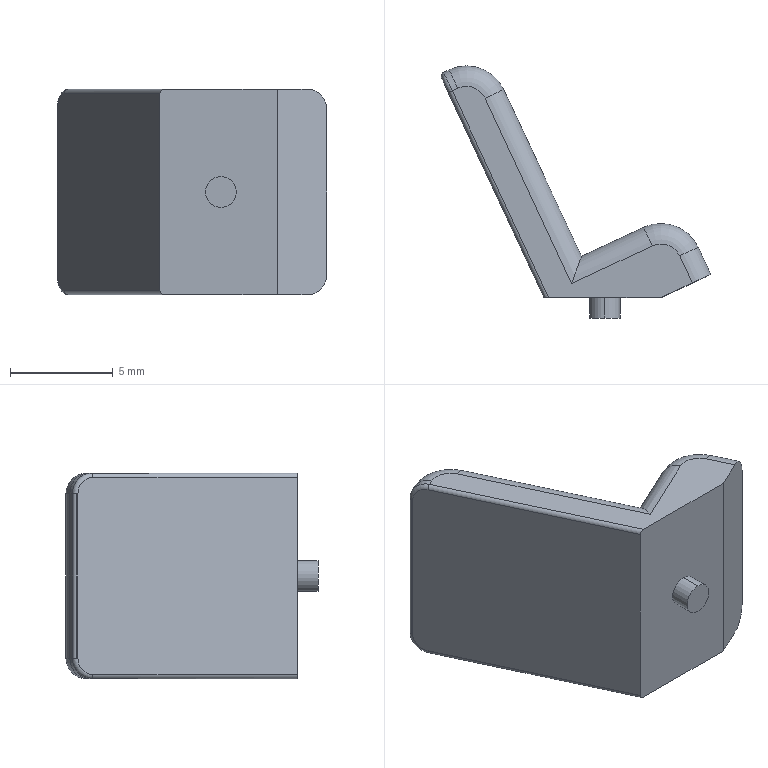Part | SolidWorks | features Fillet 2, Extrusion 1, ICE 1 | 1 solid | 32 faces | box 13.131 x 12.274 x 10 mm | volume 457.95 mm3 | cylinder 16 | plane 10 | torus 6 | commonest cylinder face diameters 2 x8 0.4 x4 1.5 x2 4 x2
STEP:
#1=CARTESIAN_POINT('',(2.965,-1.,-0.75));
#2=VERTEX_POINT('',#1);
#3=CARTESIAN_POINT('',(2.965,-1.,0.75));
#4=VERTEX_POINT('',#3);
#5=CARTESIAN_POINT('',(2.965,-1.,0.));
#6=DIRECTION('',(0.,-1.,0.));
#7=DIRECTION('',(0.,0.,-1.));
#8=AXIS2_PLACEMENT_3D('',#5,#6,#7);
#9=CIRCLE('',#8,0.75);
#10=EDGE_CURVE('',#2,#4,#9,.T.);
#11=ORIENTED_EDGE('',*,*,#10,.F.);
#12=CARTESIAN_POINT('',(2.965,0.,-0.75));
#13=VERTEX_POINT('',#12);
#14=CARTESIAN_POINT('',(2.965,-1.,-0.75));
#15=DIRECTION('',(0.,1.,0.));
#16=VECTOR('',#15,1000.);
#17=LINE('',#14,#16);
#18=EDGE_CURVE('',#2,#13,#17,.T.);
#19=ORIENTED_EDGE('',*,*,#18,.T.);
#20=CARTESIAN_POINT('',(2.965,0.,0.75));
#21=VERTEX_POINT('',#20);
#22=CARTESIAN_POINT('',(2.965,0.,0.));
#23=DIRECTION('',(0.,-1.,0.));
#24=DIRECTION('',(0.,0.,1.));
#25=AXIS2_PLACEMENT_3D('',#22,#23,#24);
#26=CIRCLE('',#25,0.75);
#27=EDGE_CURVE('',#13,#21,#26,.T.);
#28=ORIENTED_EDGE('',*,*,#27,.T.);
#29=CARTESIAN_POINT('',(2.965,-1.,0.75));
#30=DIRECTION('',(0.,1.,0.));
#31=VECTOR('',#30,1000.);
#32=LINE('',#29,#31);
#33=EDGE_CURVE('',#4,#21,#32,.T.);
#34=ORIENTED_EDGE('',*,*,#33,.F.);
#35=EDGE_LOOP('',(#11,#19,#28,#34));
#36=FACE_OUTER_BOUND('',#35,.T.);
#37=CARTESIAN_POINT('',(2.965,-1.,0.));
#38=DIRECTION('',(0.,1.,0.));
#39=DIRECTION('',(0.,0.,1.));
#40=AXIS2_PLACEMENT_3D('',#37,#38,#39);
#41=CYLINDRICAL_SURFACE('',#40,0.75);
#42=ADVANCED_FACE('',(#36),#41,.T.);
#43=CARTESIAN_POINT('',(-4.987,10.694,4.));
#44=VERTEX_POINT('',#43);
#45=CARTESIAN_POINT('',(-5.006,10.779,4.));
#46=VERTEX_POINT('',#45);
#47=CARTESIAN_POINT('',(-4.806,10.779,4.));
#48=DIRECTION('',(0.,0.,-1.));
#49=DIRECTION('',(-1.,0.,0.));
#50=AXIS2_PLACEMENT_3D('',#47,#48,#49);
#51=CIRCLE('',#50,0.2);
#52=EDGE_CURVE('',#44,#46,#51,.T.);
#53=ORIENTED_EDGE('',*,*,#52,.T.);
#54=CARTESIAN_POINT('',(-5.006,10.779,-4.));
#55=VERTEX_POINT('',#54);
#56=CARTESIAN_POINT('',(-5.006,10.779,5.));
#57=DIRECTION('',(0.,0.,-1.));
#58=VECTOR('',#57,1000.);
#59=LINE('',#56,#58);
#60=EDGE_CURVE('',#46,#55,#59,.T.);
#61=ORIENTED_EDGE('',*,*,#60,.T.);
#62=CARTESIAN_POINT('',(-4.987,10.694,-4.));
#63=VERTEX_POINT('',#62);
#64=CARTESIAN_POINT('',(-4.806,10.779,-4.));
#65=DIRECTION('',(0.,0.,1.));
#66=DIRECTION('',(1.,0.,0.));
#67=AXIS2_PLACEMENT_3D('',#64,#65,#66);
#68=CIRCLE('',#67,0.2);
#69=EDGE_CURVE('',#55,#63,#68,.T.);
#70=ORIENTED_EDGE('',*,*,#69,.T.);
#71=CARTESIAN_POINT('',(-4.987,10.694,5.));
#72=DIRECTION('',(0.,0.,-1.));
#73=VECTOR('',#72,1000.);
#74=LINE('',#71,#73);
#75=EDGE_CURVE('',#44,#63,#74,.T.);
#76=ORIENTED_EDGE('',*,*,#75,.F.);
#77=EDGE_LOOP('',(#53,#61,#70,#76));
#78=FACE_OUTER_BOUND('',#77,.T.);
#79=CARTESIAN_POINT('',(-4.806,10.779,5.));
#80=DIRECTION('',(0.,0.,-1.));
#81=DIRECTION('',(-1.,0.,0.));
#82=AXIS2_PLACEMENT_3D('',#79,#80,#81);
#83=CYLINDRICAL_SURFACE('',#82,0.2);
#84=ADVANCED_FACE('',(#78),#83,.T.);
#85=CARTESIAN_POINT('',(-4.649,9.969,4.8));
#86=VERTEX_POINT('',#85);
#87=CARTESIAN_POINT('',(-4.649,9.969,4.));
#88=DIRECTION('',(0.9063,0.4226,0.));
#89=DIRECTION('',(-0.4226,0.9063,0.));
#90=AXIS2_PLACEMENT_3D('',#87,#88,#89);
#91=CIRCLE('',#90,0.8);
#92=EDGE_CURVE('',#44,#86,#91,.T.);
#93=ORIENTED_EDGE('',*,*,#92,.F.);
#94=ORIENTED_EDGE('',*,*,#75,.T.);
#95=CARTESIAN_POINT('',(-4.649,9.969,-4.8));
#96=VERTEX_POINT('',#95);
#97=CARTESIAN_POINT('',(-4.649,9.969,-4.));
#98=DIRECTION('',(0.9063,0.4226,0.));
#99=DIRECTION('',(-0.4226,0.9063,0.));
#100=AXIS2_PLACEMENT_3D('',#97,#98,#99);
#101=CIRCLE('',#100,0.8);
#102=EDGE_CURVE('',#96,#63,#101,.T.);
#103=ORIENTED_EDGE('',*,*,#102,.F.);
#104=CARTESIAN_POINT('',(0.,0.,-4.8));
#105=VERTEX_POINT('',#104);
#106=CARTESIAN_POINT('',(0.,0.,-4.8));
#107=DIRECTION('',(0.4226,-0.9063,0.));
#108=VECTOR('',#107,1000.);
#109=LINE('',#106,#108);
#110=EDGE_CURVE('',#96,#105,#109,.T.);
#111=ORIENTED_EDGE('',*,*,#110,.T.);
#112=CARTESIAN_POINT('',(0.,0.,4.8));
#113=VERTEX_POINT('',#112);
#114=CARTESIAN_POINT('',(0.,0.,5.));
#115=DIRECTION('',(0.,0.,-1.));
#116=VECTOR('',#115,1000.);
#117=LINE('',#114,#116);
#118=EDGE_CURVE('',#113,#105,#117,.T.);
#119=ORIENTED_EDGE('',*,*,#118,.F.);
#120=CARTESIAN_POINT('',(-5.071,10.876,4.8));
#121=DIRECTION('',(-0.4226,0.9063,0.));
#122=VECTOR('',#121,1000.);
#123=LINE('',#120,#122);
#124=EDGE_CURVE('',#113,#86,#123,.T.);
#125=ORIENTED_EDGE('',*,*,#124,.T.);
#126=EDGE_LOOP('',(#93,#94,#103,#111,#119,#125));
#127=FACE_OUTER_BOUND('',#126,.T.);
#128=CARTESIAN_POINT('',(0.,0.,5.));
#129=DIRECTION('',(0.9063,0.4226,0.));
#130=DIRECTION('',(-0.4226,0.9063,0.));
#131=AXIS2_PLACEMENT_3D('',#128,#129,#130);
#132=PLANE('',#131);
#133=ADVANCED_FACE('',(#127),#132,.F.);
#134=CARTESIAN_POINT('',(2.965,0.,0.));
#135=DIRECTION('',(0.,-1.,0.));
#136=DIRECTION('',(0.,0.,1.));
#137=AXIS2_PLACEMENT_3D('',#134,#135,#136);
#138=CIRCLE('',#137,0.75);
#139=EDGE_CURVE('',#21,#13,#138,.T.);
#140=ORIENTED_EDGE('',*,*,#139,.F.);
#141=ORIENTED_EDGE('',*,*,#27,.F.);
#142=EDGE_LOOP('',(#140,#141));
#143=FACE_BOUND('',#142,.T.);
#144=ORIENTED_EDGE('',*,*,#118,.T.);
#145=CARTESIAN_POINT('',(0.2207,0.,-5.));
#146=VERTEX_POINT('',#145);
#147=CARTESIAN_POINT('',(0.,0.,-4.8));
#148=CARTESIAN_POINT('',(0.,0.,-4.917));
#149=CARTESIAN_POINT('',(0.09141,0.,-5.));
#150=CARTESIAN_POINT('',(0.2207,0.,-5.));
#151=(BOUNDED_CURVE()B_SPLINE_CURVE(3,(#147,#148,#149,#150),.UNSPECIFIED.,.F.,.F.)B_SPLINE_CURVE_WITH_KNOTS((4,4),(3.142,4.712),.UNSPECIFIED.)CURVE()GEOMETRIC_REPRESENTATION_ITEM()RATIONAL_B_SPLINE_CURVE((1.,0.8047,0.8047,1.))REPRESENTATION_ITEM(''));
#152=EDGE_CURVE('',#105,#146,#151,.T.);
#153=ORIENTED_EDGE('',*,*,#152,.T.);
#154=CARTESIAN_POINT('',(5.71,0.,-5.));
#155=VERTEX_POINT('',#154);
#156=CARTESIAN_POINT('',(0.,0.,-5.));
#157=DIRECTION('',(1.,0.,0.));
#158=VECTOR('',#157,1000.);
#159=LINE('',#156,#158);
#160=EDGE_CURVE('',#146,#155,#159,.T.);
#161=ORIENTED_EDGE('',*,*,#160,.T.);
#162=CARTESIAN_POINT('',(5.71,0.,5.));
#163=VERTEX_POINT('',#162);
#164=CARTESIAN_POINT('',(5.71,0.,5.));
#165=DIRECTION('',(0.,0.,-1.));
#166=VECTOR('',#165,1000.);
#167=LINE('',#164,#166);
#168=EDGE_CURVE('',#163,#155,#167,.T.);
#169=ORIENTED_EDGE('',*,*,#168,.F.);
#170=CARTESIAN_POINT('',(0.2207,0.,5.));
#171=VERTEX_POINT('',#170);
#172=CARTESIAN_POINT('',(0.,0.,5.));
#173=DIRECTION('',(1.,0.,0.));
#174=VECTOR('',#173,1000.);
#175=LINE('',#172,#174);
#176=EDGE_CURVE('',#171,#163,#175,.T.);
#177=ORIENTED_EDGE('',*,*,#176,.F.);
#178=CARTESIAN_POINT('',(0.2207,0.,5.));
#179=CARTESIAN_POINT('',(0.09141,0.,5.));
#180=CARTESIAN_POINT('',(0.,0.,4.917));
#181=CARTESIAN_POINT('',(0.,0.,4.8));
#182=(BOUNDED_CURVE()B_SPLINE_CURVE(3,(#178,#179,#180,#181),.UNSPECIFIED.,.F.,.T.)B_SPLINE_CURVE_WITH_KNOTS((4,4),(4.712,6.283),.UNSPECIFIED.)CURVE()GEOMETRIC_REPRESENTATION_ITEM()RATIONAL_B_SPLINE_CURVE((1.,0.8047,0.8047,1.))REPRESENTATION_ITEM(''));
#183=EDGE_CURVE('',#171,#113,#182,.T.);
#184=ORIENTED_EDGE('',*,*,#183,.T.);
#185=EDGE_LOOP('',(#144,#153,#161,#169,#177,#184));
#186=FACE_OUTER_BOUND('',#185,.T.);
#187=CARTESIAN_POINT('',(0.,0.,5.));
#188=DIRECTION('',(0.,1.,0.));
#189=DIRECTION('',(0.,0.,1.));
#190=AXIS2_PLACEMENT_3D('',#187,#188,#189);
#191=PLANE('',#190);
#192=ADVANCED_FACE('',(#143,#186),#191,.F.);
#193=CARTESIAN_POINT('',(7.219,0.7037,-5.));
#194=VERTEX_POINT('',#193);
#195=CARTESIAN_POINT('',(5.71,0.,-5.));
#196=DIRECTION('',(0.9063,0.4226,0.));
#197=VECTOR('',#196,1000.);
#198=LINE('',#195,#197);
#199=EDGE_CURVE('',#155,#194,#198,.T.);
#200=ORIENTED_EDGE('',*,*,#199,.T.);
#201=CARTESIAN_POINT('',(8.125,1.126,-4.));
#202=VERTEX_POINT('',#201);
#203=CARTESIAN_POINT('',(7.219,0.7037,-4.));
#204=DIRECTION('',(0.4226,-0.9063,0.));
#205=DIRECTION('',(-0.9063,-0.4226,0.));
#206=AXIS2_PLACEMENT_3D('',#203,#204,#205);
#207=CIRCLE('',#206,1.);
#208=EDGE_CURVE('',#194,#202,#207,.T.);
#209=ORIENTED_EDGE('',*,*,#208,.T.);
#210=CARTESIAN_POINT('',(8.125,1.126,4.));
#211=VERTEX_POINT('',#210);
#212=CARTESIAN_POINT('',(8.125,1.126,5.));
#213=DIRECTION('',(0.,0.,-1.));
#214=VECTOR('',#213,1000.);
#215=LINE('',#212,#214);
#216=EDGE_CURVE('',#211,#202,#215,.T.);
#217=ORIENTED_EDGE('',*,*,#216,.F.);
#218=CARTESIAN_POINT('',(7.219,0.7037,5.));
#219=VERTEX_POINT('',#218);
#220=CARTESIAN_POINT('',(7.219,0.7037,4.));
#221=DIRECTION('',(0.4226,-0.9063,0.));
#222=DIRECTION('',(-0.9063,-0.4226,0.));
#223=AXIS2_PLACEMENT_3D('',#220,#221,#222);
#224=CIRCLE('',#223,1.);
#225=EDGE_CURVE('',#211,#219,#224,.T.);
#226=ORIENTED_EDGE('',*,*,#225,.T.);
#227=CARTESIAN_POINT('',(5.71,0.,5.));
#228=DIRECTION('',(0.9063,0.4226,0.));
#229=VECTOR('',#228,1000.);
#230=LINE('',#227,#229);
#231=EDGE_CURVE('',#163,#219,#230,.T.);
#232=ORIENTED_EDGE('',*,*,#231,.F.);
#233=ORIENTED_EDGE('',*,*,#168,.T.);
#234=EDGE_LOOP('',(#200,#209,#217,#226,#232,#233));
#235=FACE_OUTER_BOUND('',#234,.T.);
#236=CARTESIAN_POINT('',(5.71,0.,5.));
#237=DIRECTION('',(-0.4226,0.9063,0.));
#238=DIRECTION('',(-0.9063,-0.4226,0.));
#239=AXIS2_PLACEMENT_3D('',#236,#237,#238);
#240=PLANE('',#239);
#241=ADVANCED_FACE('',(#235),#240,.F.);
#242=ORIENTED_EDGE('',*,*,#216,.T.);
#243=CARTESIAN_POINT('',(7.511,2.444,-4.));
#244=VERTEX_POINT('',#243);
#245=CARTESIAN_POINT('',(8.125,1.126,-4.));
#246=DIRECTION('',(-0.4226,0.9063,0.));
#247=VECTOR('',#246,1000.);
#248=LINE('',#245,#247);
#249=EDGE_CURVE('',#202,#244,#248,.T.);
#250=ORIENTED_EDGE('',*,*,#249,.T.);
#251=CARTESIAN_POINT('',(7.511,2.444,4.));
#252=VERTEX_POINT('',#251);
#253=CARTESIAN_POINT('',(7.511,2.444,5.));
#254=DIRECTION('',(0.,0.,-1.));
#255=VECTOR('',#254,1000.);
#256=LINE('',#253,#255);
#257=EDGE_CURVE('',#252,#244,#256,.T.);
#258=ORIENTED_EDGE('',*,*,#257,.F.);
#259=CARTESIAN_POINT('',(8.125,1.126,4.));
#260=DIRECTION('',(0.4226,-0.9063,0.));
#261=VECTOR('',#260,1000.);
#262=LINE('',#259,#261);
#263=EDGE_CURVE('',#252,#211,#262,.T.);
#264=ORIENTED_EDGE('',*,*,#263,.T.);
#265=EDGE_LOOP('',(#242,#250,#258,#264));
#266=FACE_OUTER_BOUND('',#265,.T.);
#267=CARTESIAN_POINT('',(8.125,1.126,5.));
#268=DIRECTION('',(-0.9063,-0.4226,0.));
#269=DIRECTION('',(0.4226,-0.9063,0.));
#270=AXIS2_PLACEMENT_3D('',#267,#268,#269);
#271=PLANE('',#270);
#272=ADVANCED_FACE('',(#266),#271,.F.);
#273=ORIENTED_EDGE('',*,*,#257,.T.);
#274=CARTESIAN_POINT('',(4.853,3.412,-4.));
#275=VERTEX_POINT('',#274);
#276=CARTESIAN_POINT('',(5.698,1.599,-4.));
#277=DIRECTION('',(0.,0.,1.));
#278=DIRECTION('',(1.,0.,0.));
#279=AXIS2_PLACEMENT_3D('',#276,#277,#278);
#280=CIRCLE('',#279,2.);
#281=EDGE_CURVE('',#244,#275,#280,.T.);
#282=ORIENTED_EDGE('',*,*,#281,.T.);
#283=CARTESIAN_POINT('',(4.853,3.412,4.));
#284=VERTEX_POINT('',#283);
#285=CARTESIAN_POINT('',(4.853,3.412,5.));
#286=DIRECTION('',(0.,0.,-1.));
#287=VECTOR('',#286,1000.);
#288=LINE('',#285,#287);
#289=EDGE_CURVE('',#284,#275,#288,.T.);
#290=ORIENTED_EDGE('',*,*,#289,.F.);
#291=CARTESIAN_POINT('',(5.698,1.599,4.));
#292=DIRECTION('',(0.,0.,-1.));
#293=DIRECTION('',(1.,0.,0.));
#294=AXIS2_PLACEMENT_3D('',#291,#292,#293);
#295=CIRCLE('',#294,2.);
#296=EDGE_CURVE('',#284,#252,#295,.T.);
#297=ORIENTED_EDGE('',*,*,#296,.T.);
#298=EDGE_LOOP('',(#273,#282,#290,#297));
#299=FACE_OUTER_BOUND('',#298,.T.);
#300=CARTESIAN_POINT('',(5.698,1.599,5.));
#301=DIRECTION('',(0.,0.,-1.));
#302=DIRECTION('',(-1.,0.,0.));
#303=AXIS2_PLACEMENT_3D('',#300,#301,#302);
#304=CYLINDRICAL_SURFACE('',#303,2.);
#305=ADVANCED_FACE('',(#299),#304,.T.);
#306=ORIENTED_EDGE('',*,*,#289,.T.);
#307=CARTESIAN_POINT('',(1.826,2.,-4.));
#308=VERTEX_POINT('',#307);
#309=CARTESIAN_POINT('',(4.853,3.412,-4.));
#310=DIRECTION('',(-0.9063,-0.4226,0.));
#311=VECTOR('',#310,1000.);
#312=LINE('',#309,#311);
#313=EDGE_CURVE('',#275,#308,#312,.T.);
#314=ORIENTED_EDGE('',*,*,#313,.T.);
#315=CARTESIAN_POINT('',(1.826,2.,4.));
#316=VERTEX_POINT('',#315);
#317=CARTESIAN_POINT('',(1.826,2.,5.));
#318=DIRECTION('',(0.,0.,-1.));
#319=VECTOR('',#318,1000.);
#320=LINE('',#317,#319);
#321=EDGE_CURVE('',#316,#308,#320,.T.);
#322=ORIENTED_EDGE('',*,*,#321,.F.);
#323=CARTESIAN_POINT('',(4.853,3.412,4.));
#324=DIRECTION('',(0.9063,0.4226,0.));
#325=VECTOR('',#324,1000.);
#326=LINE('',#323,#325);
#327=EDGE_CURVE('',#316,#284,#326,.T.);
#328=ORIENTED_EDGE('',*,*,#327,.T.);
#329=EDGE_LOOP('',(#306,#314,#322,#328));
#330=FACE_OUTER_BOUND('',#329,.T.);
#331=CARTESIAN_POINT('',(4.853,3.412,5.));
#332=DIRECTION('',(0.4226,-0.9063,0.));
#333=DIRECTION('',(0.9063,0.4226,0.));
#334=AXIS2_PLACEMENT_3D('',#331,#332,#333);
#335=PLANE('',#334);
#336=ADVANCED_FACE('',(#330),#335,.F.);
#337=ORIENTED_EDGE('',*,*,#321,.T.);
#338=CARTESIAN_POINT('',(-1.96,10.12,-4.));
#339=VERTEX_POINT('',#338);
#340=CARTESIAN_POINT('',(1.826,2.,-4.));
#341=DIRECTION('',(-0.4226,0.9063,0.));
#342=VECTOR('',#341,1000.);
#343=LINE('',#340,#342);
#344=EDGE_CURVE('',#308,#339,#343,.T.);
#345=ORIENTED_EDGE('',*,*,#344,.T.);
#346=CARTESIAN_POINT('',(-1.96,10.12,4.));
#347=VERTEX_POINT('',#346);
#348=CARTESIAN_POINT('',(-1.96,10.12,5.));
#349=DIRECTION('',(0.,0.,-1.));
#350=VECTOR('',#349,1000.);
#351=LINE('',#348,#350);
#352=EDGE_CURVE('',#347,#339,#351,.T.);
#353=ORIENTED_EDGE('',*,*,#352,.F.);
#354=CARTESIAN_POINT('',(1.826,2.,4.));
#355=DIRECTION('',(0.4226,-0.9063,0.));
#356=VECTOR('',#355,1000.);
#357=LINE('',#354,#356);
#358=EDGE_CURVE('',#347,#316,#357,.T.);
#359=ORIENTED_EDGE('',*,*,#358,.T.);
#360=EDGE_LOOP('',(#337,#345,#353,#359));
#361=FACE_OUTER_BOUND('',#360,.T.);
#362=CARTESIAN_POINT('',(1.826,2.,5.));
#363=DIRECTION('',(-0.9063,-0.4226,0.));
#364=DIRECTION('',(0.4226,-0.9063,0.));
#365=AXIS2_PLACEMENT_3D('',#362,#363,#364);
#366=PLANE('',#365);
#367=ADVANCED_FACE('',(#361),#366,.F.);
#368=ORIENTED_EDGE('',*,*,#352,.T.);
#369=CARTESIAN_POINT('',(-4.618,11.087,-4.));
#370=VERTEX_POINT('',#369);
#371=CARTESIAN_POINT('',(-3.773,9.274,-4.));
#372=DIRECTION('',(0.,0.,1.));
#373=DIRECTION('',(1.,0.,0.));
#374=AXIS2_PLACEMENT_3D('',#371,#372,#373);
#375=CIRCLE('',#374,2.);
#376=EDGE_CURVE('',#339,#370,#375,.T.);
#377=ORIENTED_EDGE('',*,*,#376,.T.);
#378=CARTESIAN_POINT('',(-4.618,11.087,4.));
#379=VERTEX_POINT('',#378);
#380=CARTESIAN_POINT('',(-4.618,11.087,5.));
#381=DIRECTION('',(0.,0.,-1.));
#382=VECTOR('',#381,1000.);
#383=LINE('',#380,#382);
#384=EDGE_CURVE('',#379,#370,#383,.T.);
#385=ORIENTED_EDGE('',*,*,#384,.F.);
#386=CARTESIAN_POINT('',(-3.773,9.274,4.));
#387=DIRECTION('',(0.,0.,-1.));
#388=DIRECTION('',(1.,0.,0.));
#389=AXIS2_PLACEMENT_3D('',#386,#387,#388);
#390=CIRCLE('',#389,2.);
#391=EDGE_CURVE('',#379,#347,#390,.T.);
#392=ORIENTED_EDGE('',*,*,#391,.T.);
#393=EDGE_LOOP('',(#368,#377,#385,#392));
#394=FACE_OUTER_BOUND('',#393,.T.);
#395=CARTESIAN_POINT('',(-3.773,9.274,5.));
#396=DIRECTION('',(0.,0.,-1.));
#397=DIRECTION('',(-1.,0.,0.));
#398=AXIS2_PLACEMENT_3D('',#395,#396,#397);
#399=CYLINDRICAL_SURFACE('',#398,2.);
#400=ADVANCED_FACE('',(#394),#399,.T.);
#401=ORIENTED_EDGE('',*,*,#384,.T.);
#402=CARTESIAN_POINT('',(-4.89,10.96,-4.));
#403=VERTEX_POINT('',#402);
#404=CARTESIAN_POINT('',(-4.618,11.087,-4.));
#405=DIRECTION('',(-0.9063,-0.4226,0.));
#406=VECTOR('',#405,1000.);
#407=LINE('',#404,#406);
#408=EDGE_CURVE('',#370,#403,#407,.T.);
#409=ORIENTED_EDGE('',*,*,#408,.T.);
#410=CARTESIAN_POINT('',(-4.89,10.96,4.));
#411=VERTEX_POINT('',#410);
#412=CARTESIAN_POINT('',(-4.89,10.96,5.));
#413=DIRECTION('',(0.,0.,1.));
#414=VECTOR('',#413,1000.);
#415=LINE('',#412,#414);
#416=EDGE_CURVE('',#403,#411,#415,.T.);
#417=ORIENTED_EDGE('',*,*,#416,.T.);
#418=CARTESIAN_POINT('',(-4.618,11.087,4.));
#419=DIRECTION('',(0.9063,0.4226,0.));
#420=VECTOR('',#419,1000.);
#421=LINE('',#418,#420);
#422=EDGE_CURVE('',#411,#379,#421,.T.);
#423=ORIENTED_EDGE('',*,*,#422,.T.);
#424=EDGE_LOOP('',(#401,#409,#417,#423));
#425=FACE_OUTER_BOUND('',#424,.T.);
#426=CARTESIAN_POINT('',(-4.618,11.087,5.));
#427=DIRECTION('',(0.4226,-0.9063,0.));
#428=DIRECTION('',(0.9063,0.4226,0.));
#429=AXIS2_PLACEMENT_3D('',#426,#427,#428);
#430=PLANE('',#429);
#431=ADVANCED_FACE('',(#425),#430,.F.);
#432=CARTESIAN_POINT('',(-2.867,9.697,5.));
#433=VERTEX_POINT('',#432);
#434=CARTESIAN_POINT('',(-4.196,10.181,5.));
#435=VERTEX_POINT('',#434);
#436=CARTESIAN_POINT('',(-3.773,9.274,5.));
#437=DIRECTION('',(0.,0.,1.));
#438=DIRECTION('',(1.,0.,0.));
#439=AXIS2_PLACEMENT_3D('',#436,#437,#438);
#440=CIRCLE('',#439,1.);
#441=EDGE_CURVE('',#433,#435,#440,.T.);
#442=ORIENTED_EDGE('',*,*,#441,.T.);
#443=CARTESIAN_POINT('',(-4.468,10.054,5.));
#444=VERTEX_POINT('',#443);
#445=CARTESIAN_POINT('',(-4.468,10.054,5.));
#446=DIRECTION('',(-0.9063,-0.4226,0.));
#447=VECTOR('',#446,1000.);
#448=LINE('',#445,#447);
#449=EDGE_CURVE('',#435,#444,#448,.T.);
#450=ORIENTED_EDGE('',*,*,#449,.T.);
#451=CARTESIAN_POINT('',(0.1813,0.08452,5.));
#452=DIRECTION('',(0.4226,-0.9063,0.));
#453=VECTOR('',#452,1000.);
#454=LINE('',#451,#453);
#455=EDGE_CURVE('',#444,#171,#454,.T.);
#456=ORIENTED_EDGE('',*,*,#455,.T.);
#457=ORIENTED_EDGE('',*,*,#176,.T.);
#458=ORIENTED_EDGE('',*,*,#231,.T.);
#459=CARTESIAN_POINT('',(6.604,2.022,5.));
#460=VERTEX_POINT('',#459);
#461=CARTESIAN_POINT('',(6.604,2.022,5.));
#462=DIRECTION('',(-0.4226,0.9063,0.));
#463=VECTOR('',#462,1000.);
#464=LINE('',#461,#463);
#465=EDGE_CURVE('',#219,#460,#464,.T.);
#466=ORIENTED_EDGE('',*,*,#465,.T.);
#467=CARTESIAN_POINT('',(5.276,2.505,5.));
#468=VERTEX_POINT('',#467);
#469=CARTESIAN_POINT('',(5.698,1.599,5.));
#470=DIRECTION('',(0.,0.,1.));
#471=DIRECTION('',(1.,0.,0.));
#472=AXIS2_PLACEMENT_3D('',#469,#470,#471);
#473=CIRCLE('',#472,1.);
#474=EDGE_CURVE('',#460,#468,#473,.T.);
#475=ORIENTED_EDGE('',*,*,#474,.T.);
#476=CARTESIAN_POINT('',(1.342,0.6711,5.));
#477=VERTEX_POINT('',#476);
#478=CARTESIAN_POINT('',(2.248,1.094,5.));
#479=DIRECTION('',(-0.9063,-0.4226,0.));
#480=VECTOR('',#479,1000.);
#481=LINE('',#478,#480);
#482=EDGE_CURVE('',#468,#477,#481,.T.);
#483=ORIENTED_EDGE('',*,*,#482,.T.);
#484=CARTESIAN_POINT('',(-2.867,9.697,5.));
#485=DIRECTION('',(-0.4226,0.9063,0.));
#486=VECTOR('',#485,1000.);
#487=LINE('',#484,#486);
#488=EDGE_CURVE('',#477,#433,#487,.T.);
#489=ORIENTED_EDGE('',*,*,#488,.T.);
#490=EDGE_LOOP('',(#442,#450,#456,#457,#458,#466,#475,#483,#489));
#491=FACE_OUTER_BOUND('',#490,.T.);
#492=CARTESIAN_POINT('',(5.698,1.599,5.));
#493=DIRECTION('',(0.,0.,1.));
#494=DIRECTION('',(1.,0.,0.));
#495=AXIS2_PLACEMENT_3D('',#492,#493,#494);
#496=PLANE('',#495);
#497=ADVANCED_FACE('',(#491),#496,.T.);
#498=CARTESIAN_POINT('',(5.276,2.505,-5.));
#499=VERTEX_POINT('',#498);
#500=CARTESIAN_POINT('',(6.604,2.022,-5.));
#501=VERTEX_POINT('',#500);
#502=CARTESIAN_POINT('',(5.698,1.599,-5.));
#503=DIRECTION('',(0.,0.,-1.));
#504=DIRECTION('',(1.,0.,0.));
#505=AXIS2_PLACEMENT_3D('',#502,#503,#504);
#506=CIRCLE('',#505,1.);
#507=EDGE_CURVE('',#499,#501,#506,.T.);
#508=ORIENTED_EDGE('',*,*,#507,.T.);
#509=CARTESIAN_POINT('',(6.604,2.022,-5.));
#510=DIRECTION('',(0.4226,-0.9063,0.));
#511=VECTOR('',#510,1000.);
#512=LINE('',#509,#511);
#513=EDGE_CURVE('',#501,#194,#512,.T.);
#514=ORIENTED_EDGE('',*,*,#513,.T.);
#515=ORIENTED_EDGE('',*,*,#199,.F.);
#516=ORIENTED_EDGE('',*,*,#160,.F.);
#517=CARTESIAN_POINT('',(-4.468,10.054,-5.));
#518=VERTEX_POINT('',#517);
#519=CARTESIAN_POINT('',(0.5866,-0.7846,-5.));
#520=DIRECTION('',(-0.4226,0.9063,0.));
#521=VECTOR('',#520,1000.);
#522=LINE('',#519,#521);
#523=EDGE_CURVE('',#146,#518,#522,.T.);
#524=ORIENTED_EDGE('',*,*,#523,.T.);
#525=CARTESIAN_POINT('',(-4.196,10.181,-5.));
#526=VERTEX_POINT('',#525);
#527=CARTESIAN_POINT('',(0.644,12.437,-5.));
#528=DIRECTION('',(0.9063,0.4226,0.));
#529=VECTOR('',#528,1000.);
#530=LINE('',#527,#529);
#531=EDGE_CURVE('',#518,#526,#530,.T.);
#532=ORIENTED_EDGE('',*,*,#531,.T.);
#533=CARTESIAN_POINT('',(-2.867,9.697,-5.));
#534=VERTEX_POINT('',#533);
#535=CARTESIAN_POINT('',(-3.773,9.274,-5.));
#536=DIRECTION('',(0.,0.,-1.));
#537=DIRECTION('',(1.,0.,0.));
#538=AXIS2_PLACEMENT_3D('',#535,#536,#537);
#539=CIRCLE('',#538,1.);
#540=EDGE_CURVE('',#526,#534,#539,.T.);
#541=ORIENTED_EDGE('',*,*,#540,.T.);
#542=CARTESIAN_POINT('',(1.342,0.6711,-5.));
#543=VERTEX_POINT('',#542);
#544=CARTESIAN_POINT('',(1.765,-0.2352,-5.));
#545=DIRECTION('',(0.4226,-0.9063,0.));
#546=VECTOR('',#545,1000.);
#547=LINE('',#544,#546);
#548=EDGE_CURVE('',#534,#543,#547,.T.);
#549=ORIENTED_EDGE('',*,*,#548,.T.);
#550=CARTESIAN_POINT('',(5.276,2.505,-5.));
#551=DIRECTION('',(0.9063,0.4226,0.));
#552=VECTOR('',#551,1000.);
#553=LINE('',#550,#552);
#554=EDGE_CURVE('',#543,#499,#553,.T.);
#555=ORIENTED_EDGE('',*,*,#554,.T.);
#556=EDGE_LOOP('',(#508,#514,#515,#516,#524,#532,#541,#549,#555));
#557=FACE_OUTER_BOUND('',#556,.T.);
#558=CARTESIAN_POINT('',(5.698,1.599,-5.));
#559=DIRECTION('',(0.,0.,1.));
#560=DIRECTION('',(1.,0.,0.));
#561=AXIS2_PLACEMENT_3D('',#558,#559,#560);
#562=PLANE('',#561);
#563=ADVANCED_FACE('',(#557),#562,.F.);
#564=ORIENTED_EDGE('',*,*,#455,.F.);
#565=CARTESIAN_POINT('',(-4.468,10.054,4.8));
#566=DIRECTION('',(0.4226,-0.9063,0.));
#567=DIRECTION('',(0.9063,0.4226,0.));
#568=AXIS2_PLACEMENT_3D('',#565,#566,#567);
#569=CIRCLE('',#568,0.2);
#570=EDGE_CURVE('',#444,#86,#569,.T.);
#571=ORIENTED_EDGE('',*,*,#570,.T.);
#572=ORIENTED_EDGE('',*,*,#124,.F.);
#573=ORIENTED_EDGE('',*,*,#183,.F.);
#574=EDGE_LOOP('',(#564,#571,#572,#573));
#575=FACE_OUTER_BOUND('',#574,.T.);
#576=CARTESIAN_POINT('',(0.5866,-0.7846,4.8));
#577=DIRECTION('',(-0.4226,0.9063,0.));
#578=DIRECTION('',(-0.9063,-0.4226,0.));
#579=AXIS2_PLACEMENT_3D('',#576,#577,#578);
#580=CYLINDRICAL_SURFACE('',#579,0.2);
#581=ADVANCED_FACE('',(#575),#580,.T.);
#582=ORIENTED_EDGE('',*,*,#60,.F.);
#583=CARTESIAN_POINT('',(-4.806,10.779,4.));
#584=DIRECTION('',(0.,0.,-1.));
#585=DIRECTION('',(-1.,0.,0.));
#586=AXIS2_PLACEMENT_3D('',#583,#584,#585);
#587=CIRCLE('',#586,0.2);
#588=EDGE_CURVE('',#46,#411,#587,.T.);
#589=ORIENTED_EDGE('',*,*,#588,.T.);
#590=ORIENTED_EDGE('',*,*,#416,.F.);
#591=CARTESIAN_POINT('',(-4.806,10.779,-4.));
#592=DIRECTION('',(0.,0.,1.));
#593=DIRECTION('',(1.,0.,0.));
#594=AXIS2_PLACEMENT_3D('',#591,#592,#593);
#595=CIRCLE('',#594,0.2);
#596=EDGE_CURVE('',#403,#55,#595,.T.);
#597=ORIENTED_EDGE('',*,*,#596,.T.);
#598=EDGE_LOOP('',(#582,#589,#590,#597));
#599=FACE_OUTER_BOUND('',#598,.T.);
#600=CARTESIAN_POINT('',(-4.806,10.779,5.));
#601=DIRECTION('',(0.,0.,-1.));
#602=DIRECTION('',(-1.,0.,0.));
#603=AXIS2_PLACEMENT_3D('',#600,#601,#602);
#604=CYLINDRICAL_SURFACE('',#603,0.2);
#605=ADVANCED_FACE('',(#599),#604,.T.);
#606=ORIENTED_EDGE('',*,*,#110,.F.);
#607=CARTESIAN_POINT('',(-4.468,10.054,-4.8));
#608=DIRECTION('',(0.4226,-0.9063,0.));
#609=DIRECTION('',(0.9063,0.4226,0.));
#610=AXIS2_PLACEMENT_3D('',#607,#608,#609);
#611=CIRCLE('',#610,0.2);
#612=EDGE_CURVE('',#96,#518,#611,.T.);
#613=ORIENTED_EDGE('',*,*,#612,.T.);
#614=ORIENTED_EDGE('',*,*,#523,.F.);
#615=ORIENTED_EDGE('',*,*,#152,.F.);
#616=EDGE_LOOP('',(#606,#613,#614,#615));
#617=FACE_OUTER_BOUND('',#616,.T.);
#618=CARTESIAN_POINT('',(0.1813,0.08452,-4.8));
#619=DIRECTION('',(0.4226,-0.9063,0.));
#620=DIRECTION('',(0.9063,0.4226,0.));
#621=AXIS2_PLACEMENT_3D('',#618,#619,#620);
#622=CYLINDRICAL_SURFACE('',#621,0.2);
#623=ADVANCED_FACE('',(#617),#622,.T.);
#624=ORIENTED_EDGE('',*,*,#225,.F.);
#625=ORIENTED_EDGE('',*,*,#263,.F.);
#626=CARTESIAN_POINT('',(6.604,2.022,4.));
#627=DIRECTION('',(-0.4226,0.9063,0.));
#628=DIRECTION('',(-0.9063,-0.4226,0.));
#629=AXIS2_PLACEMENT_3D('',#626,#627,#628);
#630=CIRCLE('',#629,1.);
#631=EDGE_CURVE('',#460,#252,#630,.T.);
#632=ORIENTED_EDGE('',*,*,#631,.F.);
#633=ORIENTED_EDGE('',*,*,#465,.F.);
#634=EDGE_LOOP('',(#624,#625,#632,#633));
#635=FACE_OUTER_BOUND('',#634,.T.);
#636=CARTESIAN_POINT('',(6.604,2.022,4.));
#637=DIRECTION('',(0.4226,-0.9063,0.));
#638=DIRECTION('',(0.9063,0.4226,0.));
#639=AXIS2_PLACEMENT_3D('',#636,#637,#638);
#640=CYLINDRICAL_SURFACE('',#639,1.);
#641=ADVANCED_FACE('',(#635),#640,.T.);
#642=ORIENTED_EDGE('',*,*,#631,.T.);
#643=ORIENTED_EDGE('',*,*,#296,.F.);
#644=CARTESIAN_POINT('',(5.276,2.505,4.));
#645=DIRECTION('',(-0.9063,-0.4226,0.));
#646=DIRECTION('',(0.4226,-0.9063,0.));
#647=AXIS2_PLACEMENT_3D('',#644,#645,#646);
#648=CIRCLE('',#647,1.);
#649=EDGE_CURVE('',#468,#284,#648,.T.);
#650=ORIENTED_EDGE('',*,*,#649,.F.);
#651=ORIENTED_EDGE('',*,*,#474,.F.);
#652=EDGE_LOOP('',(#642,#643,#650,#651));
#653=FACE_OUTER_BOUND('',#652,.T.);
#654=CARTESIAN_POINT('',(5.698,1.599,4.));
#655=DIRECTION('',(0.,0.,1.));
#656=DIRECTION('',(1.,0.,0.));
#657=AXIS2_PLACEMENT_3D('',#654,#655,#656);
#658=TOROIDAL_SURFACE('',#657,1.,1.);
#659=ADVANCED_FACE('',(#653),#658,.T.);
#660=ORIENTED_EDGE('',*,*,#649,.T.);
#661=ORIENTED_EDGE('',*,*,#327,.F.);
#662=CARTESIAN_POINT('',(1.342,0.6711,5.));
#663=CARTESIAN_POINT('',(1.625,1.45,5.));
#664=CARTESIAN_POINT('',(1.826,2.,4.586));
#665=CARTESIAN_POINT('',(1.826,2.,4.));
#666=(BOUNDED_CURVE()B_SPLINE_CURVE(3,(#662,#663,#664,#665),.UNSPECIFIED.,.F.,.T.)B_SPLINE_CURVE_WITH_KNOTS((4,4),(1.571,3.142),.UNSPECIFIED.)CURVE()GEOMETRIC_REPRESENTATION_ITEM()RATIONAL_B_SPLINE_CURVE((1.,0.8047,0.8047,1.))REPRESENTATION_ITEM(''));
#667=EDGE_CURVE('',#477,#316,#666,.T.);
#668=ORIENTED_EDGE('',*,*,#667,.F.);
#669=ORIENTED_EDGE('',*,*,#482,.F.);
#670=EDGE_LOOP('',(#660,#661,#668,#669));
#671=FACE_OUTER_BOUND('',#670,.T.);
#672=CARTESIAN_POINT('',(5.276,2.505,4.));
#673=DIRECTION('',(0.9063,0.4226,0.));
#674=DIRECTION('',(-0.4226,0.9063,0.));
#675=AXIS2_PLACEMENT_3D('',#672,#673,#674);
#676=CYLINDRICAL_SURFACE('',#675,1.);
#677=ADVANCED_FACE('',(#671),#676,.T.);
#678=ORIENTED_EDGE('',*,*,#667,.T.);
#679=ORIENTED_EDGE('',*,*,#358,.F.);
#680=CARTESIAN_POINT('',(-2.867,9.697,4.));
#681=DIRECTION('',(-0.4226,0.9063,0.));
#682=DIRECTION('',(-0.9063,-0.4226,0.));
#683=AXIS2_PLACEMENT_3D('',#680,#681,#682);
#684=CIRCLE('',#683,1.);
#685=EDGE_CURVE('',#433,#347,#684,.T.);
#686=ORIENTED_EDGE('',*,*,#685,.F.);
#687=ORIENTED_EDGE('',*,*,#488,.F.);
#688=EDGE_LOOP('',(#678,#679,#686,#687));
#689=FACE_OUTER_BOUND('',#688,.T.);
#690=CARTESIAN_POINT('',(1.765,-0.2352,4.));
#691=DIRECTION('',(0.4226,-0.9063,0.));
#692=DIRECTION('',(0.9063,0.4226,0.));
#693=AXIS2_PLACEMENT_3D('',#690,#691,#692);
#694=CYLINDRICAL_SURFACE('',#693,1.);
#695=ADVANCED_FACE('',(#689),#694,.T.);
#696=ORIENTED_EDGE('',*,*,#685,.T.);
#697=ORIENTED_EDGE('',*,*,#391,.F.);
#698=CARTESIAN_POINT('',(-4.196,10.181,4.));
#699=DIRECTION('',(-0.9063,-0.4226,0.));
#700=DIRECTION('',(0.4226,-0.9063,0.));
#701=AXIS2_PLACEMENT_3D('',#698,#699,#700);
#702=CIRCLE('',#701,1.);
#703=EDGE_CURVE('',#435,#379,#702,.T.);
#704=ORIENTED_EDGE('',*,*,#703,.F.);
#705=ORIENTED_EDGE('',*,*,#441,.F.);
#706=EDGE_LOOP('',(#696,#697,#704,#705));
#707=FACE_OUTER_BOUND('',#706,.T.);
#708=CARTESIAN_POINT('',(-3.773,9.274,4.));
#709=DIRECTION('',(0.,0.,1.));
#710=DIRECTION('',(1.,0.,0.));
#711=AXIS2_PLACEMENT_3D('',#708,#709,#710);
#712=TOROIDAL_SURFACE('',#711,1.,1.);
#713=ADVANCED_FACE('',(#707),#712,.T.);
#714=ORIENTED_EDGE('',*,*,#703,.T.);
#715=ORIENTED_EDGE('',*,*,#422,.F.);
#716=CARTESIAN_POINT('',(-4.468,10.054,4.));
#717=DIRECTION('',(-0.9063,-0.4226,0.));
#718=DIRECTION('',(-0.4226,0.9063,0.));
#719=AXIS2_PLACEMENT_3D('',#716,#717,#718);
#720=CIRCLE('',#719,1.);
#721=EDGE_CURVE('',#444,#411,#720,.T.);
#722=ORIENTED_EDGE('',*,*,#721,.F.);
#723=ORIENTED_EDGE('',*,*,#449,.F.);
#724=EDGE_LOOP('',(#714,#715,#722,#723));
#725=FACE_OUTER_BOUND('',#724,.T.);
#726=CARTESIAN_POINT('',(0.644,12.437,4.));
#727=DIRECTION('',(0.9063,0.4226,0.));
#728=DIRECTION('',(-0.4226,0.9063,0.));
#729=AXIS2_PLACEMENT_3D('',#726,#727,#728);
#730=CYLINDRICAL_SURFACE('',#729,1.);
#731=ADVANCED_FACE('',(#725),#730,.T.);
#732=ORIENTED_EDGE('',*,*,#570,.F.);
#733=ORIENTED_EDGE('',*,*,#721,.T.);
#734=ORIENTED_EDGE('',*,*,#588,.F.);
#735=ORIENTED_EDGE('',*,*,#52,.F.);
#736=ORIENTED_EDGE('',*,*,#92,.T.);
#737=EDGE_LOOP('',(#732,#733,#734,#735,#736));
#738=FACE_OUTER_BOUND('',#737,.T.);
#739=CARTESIAN_POINT('',(-4.468,10.054,4.));
#740=DIRECTION('',(0.9063,0.4226,0.));
#741=DIRECTION('',(-0.4226,0.9063,0.));
#742=AXIS2_PLACEMENT_3D('',#739,#740,#741);
#743=TOROIDAL_SURFACE('',#742,0.8,0.2);
#744=ADVANCED_FACE('',(#738),#743,.T.);
#745=ORIENTED_EDGE('',*,*,#208,.F.);
#746=ORIENTED_EDGE('',*,*,#513,.F.);
#747=CARTESIAN_POINT('',(6.604,2.022,-4.));
#748=DIRECTION('',(-0.4226,0.9063,0.));
#749=DIRECTION('',(-0.9063,-0.4226,0.));
#750=AXIS2_PLACEMENT_3D('',#747,#748,#749);
#751=CIRCLE('',#750,1.);
#752=EDGE_CURVE('',#244,#501,#751,.T.);
#753=ORIENTED_EDGE('',*,*,#752,.F.);
#754=ORIENTED_EDGE('',*,*,#249,.F.);
#755=EDGE_LOOP('',(#745,#746,#753,#754));
#756=FACE_OUTER_BOUND('',#755,.T.);
#757=CARTESIAN_POINT('',(7.219,0.7037,-4.));
#758=DIRECTION('',(-0.4226,0.9063,0.));
#759=DIRECTION('',(-0.9063,-0.4226,0.));
#760=AXIS2_PLACEMENT_3D('',#757,#758,#759);
#761=CYLINDRICAL_SURFACE('',#760,1.);
#762=ADVANCED_FACE('',(#756),#761,.T.);
#763=ORIENTED_EDGE('',*,*,#752,.T.);
#764=ORIENTED_EDGE('',*,*,#507,.F.);
#765=CARTESIAN_POINT('',(5.276,2.505,-4.));
#766=DIRECTION('',(-0.9063,-0.4226,0.));
#767=DIRECTION('',(0.4226,-0.9063,0.));
#768=AXIS2_PLACEMENT_3D('',#765,#766,#767);
#769=CIRCLE('',#768,1.);
#770=EDGE_CURVE('',#275,#499,#769,.T.);
#771=ORIENTED_EDGE('',*,*,#770,.F.);
#772=ORIENTED_EDGE('',*,*,#281,.F.);
#773=EDGE_LOOP('',(#763,#764,#771,#772));
#774=FACE_OUTER_BOUND('',#773,.T.);
#775=CARTESIAN_POINT('',(5.698,1.599,-4.));
#776=DIRECTION('',(0.,0.,1.));
#777=DIRECTION('',(1.,0.,0.));
#778=AXIS2_PLACEMENT_3D('',#775,#776,#777);
#779=TOROIDAL_SURFACE('',#778,1.,1.);
#780=ADVANCED_FACE('',(#774),#779,.T.);
#781=ORIENTED_EDGE('',*,*,#770,.T.);
#782=ORIENTED_EDGE('',*,*,#554,.F.);
#783=CARTESIAN_POINT('',(1.826,2.,-4.));
#784=CARTESIAN_POINT('',(1.826,2.,-4.586));
#785=CARTESIAN_POINT('',(1.625,1.45,-5.));
#786=CARTESIAN_POINT('',(1.342,0.6711,-5.));
#787=(BOUNDED_CURVE()B_SPLINE_CURVE(3,(#783,#784,#785,#786),.UNSPECIFIED.,.F.,.F.)B_SPLINE_CURVE_WITH_KNOTS((4,4),(3.142,4.712),.UNSPECIFIED.)CURVE()GEOMETRIC_REPRESENTATION_ITEM()RATIONAL_B_SPLINE_CURVE((1.,0.8047,0.8047,1.))REPRESENTATION_ITEM(''));
#788=EDGE_CURVE('',#308,#543,#787,.T.);
#789=ORIENTED_EDGE('',*,*,#788,.F.);
#790=ORIENTED_EDGE('',*,*,#313,.F.);
#791=EDGE_LOOP('',(#781,#782,#789,#790));
#792=FACE_OUTER_BOUND('',#791,.T.);
#793=CARTESIAN_POINT('',(5.276,2.505,-4.));
#794=DIRECTION('',(-0.9063,-0.4226,0.));
#795=DIRECTION('',(0.4226,-0.9063,0.));
#796=AXIS2_PLACEMENT_3D('',#793,#794,#795);
#797=CYLINDRICAL_SURFACE('',#796,1.);
#798=ADVANCED_FACE('',(#792),#797,.T.);
#799=ORIENTED_EDGE('',*,*,#788,.T.);
#800=ORIENTED_EDGE('',*,*,#548,.F.);
#801=CARTESIAN_POINT('',(-2.867,9.697,-4.));
#802=DIRECTION('',(-0.4226,0.9063,0.));
#803=DIRECTION('',(-0.9063,-0.4226,0.));
#804=AXIS2_PLACEMENT_3D('',#801,#802,#803);
#805=CIRCLE('',#804,1.);
#806=EDGE_CURVE('',#339,#534,#805,.T.);
#807=ORIENTED_EDGE('',*,*,#806,.F.);
#808=ORIENTED_EDGE('',*,*,#344,.F.);
#809=EDGE_LOOP('',(#799,#800,#807,#808));
#810=FACE_OUTER_BOUND('',#809,.T.);
#811=CARTESIAN_POINT('',(0.9195,1.577,-4.));
#812=DIRECTION('',(-0.4226,0.9063,0.));
#813=DIRECTION('',(-0.9063,-0.4226,0.));
#814=AXIS2_PLACEMENT_3D('',#811,#812,#813);
#815=CYLINDRICAL_SURFACE('',#814,1.);
#816=ADVANCED_FACE('',(#810),#815,.T.);
#817=ORIENTED_EDGE('',*,*,#806,.T.);
#818=ORIENTED_EDGE('',*,*,#540,.F.);
#819=CARTESIAN_POINT('',(-4.196,10.181,-4.));
#820=DIRECTION('',(-0.9063,-0.4226,0.));
#821=DIRECTION('',(0.4226,-0.9063,0.));
#822=AXIS2_PLACEMENT_3D('',#819,#820,#821);
#823=CIRCLE('',#822,1.);
#824=EDGE_CURVE('',#370,#526,#823,.T.);
#825=ORIENTED_EDGE('',*,*,#824,.F.);
#826=ORIENTED_EDGE('',*,*,#376,.F.);
#827=EDGE_LOOP('',(#817,#818,#825,#826));
#828=FACE_OUTER_BOUND('',#827,.T.);
#829=CARTESIAN_POINT('',(-3.773,9.274,-4.));
#830=DIRECTION('',(0.,0.,1.));
#831=DIRECTION('',(1.,0.,0.));
#832=AXIS2_PLACEMENT_3D('',#829,#830,#831);
#833=TOROIDAL_SURFACE('',#832,1.,1.);
#834=ADVANCED_FACE('',(#828),#833,.T.);
#835=ORIENTED_EDGE('',*,*,#824,.T.);
#836=ORIENTED_EDGE('',*,*,#531,.F.);
#837=CARTESIAN_POINT('',(-4.468,10.054,-4.));
#838=DIRECTION('',(-0.9063,-0.4226,0.));
#839=DIRECTION('',(-0.4226,0.9063,0.));
#840=AXIS2_PLACEMENT_3D('',#837,#838,#839);
#841=CIRCLE('',#840,1.);
#842=EDGE_CURVE('',#403,#518,#841,.T.);
#843=ORIENTED_EDGE('',*,*,#842,.F.);
#844=ORIENTED_EDGE('',*,*,#408,.F.);
#845=EDGE_LOOP('',(#835,#836,#843,#844));
#846=FACE_OUTER_BOUND('',#845,.T.);
#847=CARTESIAN_POINT('',(-4.196,10.181,-4.));
#848=DIRECTION('',(-0.9063,-0.4226,0.));
#849=DIRECTION('',(0.4226,-0.9063,0.));
#850=AXIS2_PLACEMENT_3D('',#847,#848,#849);
#851=CYLINDRICAL_SURFACE('',#850,1.);
#852=ADVANCED_FACE('',(#846),#851,.T.);
#853=ORIENTED_EDGE('',*,*,#596,.F.);
#854=ORIENTED_EDGE('',*,*,#842,.T.);
#855=ORIENTED_EDGE('',*,*,#612,.F.);
#856=ORIENTED_EDGE('',*,*,#102,.T.);
#857=ORIENTED_EDGE('',*,*,#69,.F.);
#858=EDGE_LOOP('',(#853,#854,#855,#856,#857));
#859=FACE_OUTER_BOUND('',#858,.T.);
#860=CARTESIAN_POINT('',(-4.468,10.054,-4.));
#861=DIRECTION('',(0.9063,0.4226,0.));
#862=DIRECTION('',(-0.4226,0.9063,0.));
#863=AXIS2_PLACEMENT_3D('',#860,#861,#862);
#864=TOROIDAL_SURFACE('',#863,0.8,0.2);
#865=ADVANCED_FACE('',(#859),#864,.T.);
#866=ORIENTED_EDGE('',*,*,#18,.F.);
#867=CARTESIAN_POINT('',(2.965,-1.,0.));
#868=DIRECTION('',(0.,-1.,0.));
#869=DIRECTION('',(0.,0.,-1.));
#870=AXIS2_PLACEMENT_3D('',#867,#868,#869);
#871=CIRCLE('',#870,0.75);
#872=EDGE_CURVE('',#4,#2,#871,.T.);
#873=ORIENTED_EDGE('',*,*,#872,.F.);
#874=ORIENTED_EDGE('',*,*,#33,.T.);
#875=ORIENTED_EDGE('',*,*,#139,.T.);
#876=EDGE_LOOP('',(#866,#873,#874,#875));
#877=FACE_OUTER_BOUND('',#876,.T.);
#878=CARTESIAN_POINT('',(2.965,-1.,0.));
#879=DIRECTION('',(0.,1.,0.));
#880=DIRECTION('',(0.,0.,1.));
#881=AXIS2_PLACEMENT_3D('',#878,#879,#880);
#882=CYLINDRICAL_SURFACE('',#881,0.75);
#883=ADVANCED_FACE('',(#877),#882,.T.);
#884=ORIENTED_EDGE('',*,*,#872,.T.);
#885=ORIENTED_EDGE('',*,*,#10,.T.);
#886=EDGE_LOOP('',(#884,#885));
#887=FACE_OUTER_BOUND('',#886,.T.);
#888=CARTESIAN_POINT('',(2.965,-1.,0.));
#889=DIRECTION('',(0.,-1.,0.));
#890=DIRECTION('',(0.,0.,-1.));
#891=AXIS2_PLACEMENT_3D('',#888,#889,#890);
#892=PLANE('',#891);
#893=ADVANCED_FACE('',(#887),#892,.T.);
#894=CLOSED_SHELL('',(#42,#84,#133,#192,#241,#272,#305,#336,#367,#400,#431,#497,#563,#581,#605,#623,#641,#659,#677,#695,#713,#731,#744,#762,#780,#798,#816,#834,#852,#865,#883,#893));
#895=MANIFOLD_SOLID_BREP('',#894);
#896=CARTESIAN_POINT('',(0.,0.,0.));
#897=DIRECTION('',(0.,0.,1.));
#898=DIRECTION('',(1.,0.,0.));
#899=AXIS2_PLACEMENT_3D('',#896,#897,#898);
#900=(LENGTH_UNIT()NAMED_UNIT(*)SI_UNIT(.MILLI.,.METRE.));
#901=UNCERTAINTY_MEASURE_WITH_UNIT(LENGTH_MEASURE(0.00001),#900,'','');
#902=(NAMED_UNIT(*)PLANE_ANGLE_UNIT()SI_UNIT($,.RADIAN.));
#903=(NAMED_UNIT(*)SI_UNIT($,.STERADIAN.)SOLID_ANGLE_UNIT());
#904=(GEOMETRIC_REPRESENTATION_CONTEXT(3)GLOBAL_UNCERTAINTY_ASSIGNED_CONTEXT((#901))GLOBAL_UNIT_ASSIGNED_CONTEXT((#900,#902,#903))REPRESENTATION_CONTEXT('',''));
#905=ADVANCED_BREP_SHAPE_REPRESENTATION('',(#895,#899),#904);